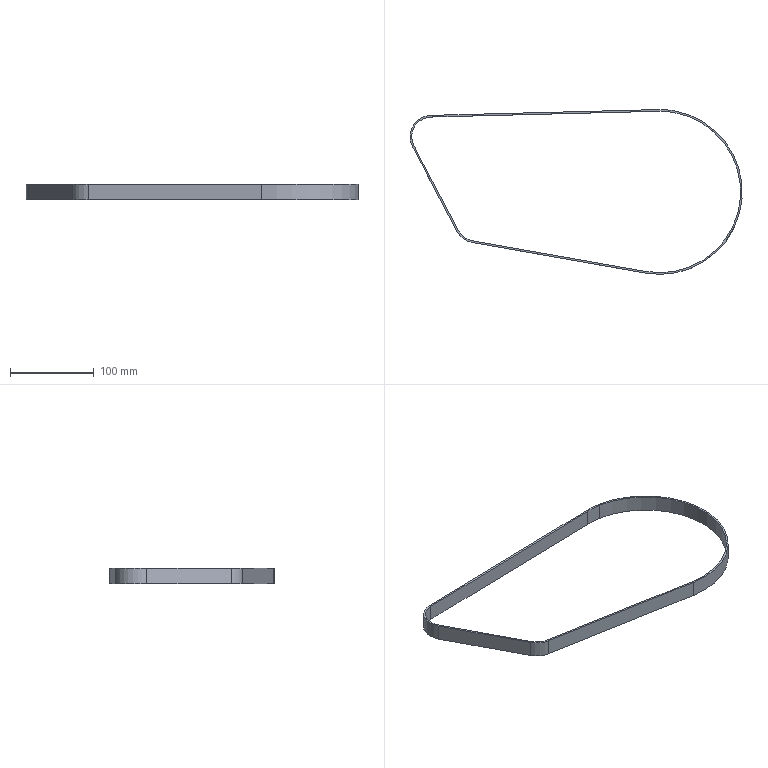Part | SolidWorks | features BaseBody 1 | 1 solid | 16 faces | box 396.622 x 196.734 x 19.05 mm | volume 38426 mm3 | cylinder 8 | plane 8 | commonest cylinder face diameters 47.139 x2 51.203 x2 192.67 x2 196.734 x2
STEP:
#1=CARTESIAN_POINT('',(270.213,30.425,-9.525));
#2=VERTEX_POINT('',#1);
#3=CARTESIAN_POINT('',(289.434,28.983,-9.525));
#4=VERTEX_POINT('',#3);
#5=CARTESIAN_POINT('',(272.654,-65.879,-9.525));
#6=DIRECTION('',(0.,0.,-1.));
#7=DIRECTION('',(0.1742,0.9847,0.));
#8=AXIS2_PLACEMENT_3D('',#5,#6,#7);
#9=CIRCLE('',#8,96.335);
#10=EDGE_CURVE('',#2,#4,#9,.T.);
#11=ORIENTED_EDGE('',*,*,#10,.T.);
#12=CARTESIAN_POINT('',(289.434,28.983,9.525));
#13=VERTEX_POINT('',#12);
#14=CARTESIAN_POINT('',(289.434,28.983,0.));
#15=DIRECTION('',(0.,0.,1.));
#16=VECTOR('',#15,1000.);
#17=LINE('',#14,#16);
#18=EDGE_CURVE('',#4,#13,#17,.T.);
#19=ORIENTED_EDGE('',*,*,#18,.T.);
#20=CARTESIAN_POINT('',(270.213,30.425,9.525));
#21=VERTEX_POINT('',#20);
#22=CARTESIAN_POINT('',(272.654,-65.879,9.525));
#23=DIRECTION('',(0.,0.,-1.));
#24=DIRECTION('',(0.1742,0.9847,0.));
#25=AXIS2_PLACEMENT_3D('',#22,#23,#24);
#26=CIRCLE('',#25,96.335);
#27=EDGE_CURVE('',#21,#13,#26,.T.);
#28=ORIENTED_EDGE('',*,*,#27,.F.);
#29=CARTESIAN_POINT('',(270.213,30.425,9.525));
#30=DIRECTION('',(0.,0.,1.));
#31=VECTOR('',#30,1000.);
#32=LINE('',#29,#31);
#33=EDGE_CURVE('',#2,#21,#32,.T.);
#34=ORIENTED_EDGE('',*,*,#33,.F.);
#35=EDGE_LOOP('',(#11,#19,#28,#34));
#36=FACE_OUTER_BOUND('',#35,.T.);
#37=CARTESIAN_POINT('',(272.654,-65.879,0.));
#38=DIRECTION('',(0.,0.,1.));
#39=DIRECTION('',(0.1742,0.9847,0.));
#40=AXIS2_PLACEMENT_3D('',#37,#38,#39);
#41=CYLINDRICAL_SURFACE('',#40,96.335);
#42=ADVANCED_FACE('',(#36),#41,.F.);
#43=CARTESIAN_POINT('',(289.788,30.984,-9.525));
#44=VERTEX_POINT('',#43);
#45=CARTESIAN_POINT('',(255.52,-162.742,-9.525));
#46=VERTEX_POINT('',#45);
#47=CARTESIAN_POINT('',(272.654,-65.879,-9.525));
#48=DIRECTION('',(0.,0.,-1.));
#49=DIRECTION('',(0.1742,0.9847,0.));
#50=AXIS2_PLACEMENT_3D('',#47,#48,#49);
#51=CIRCLE('',#50,98.367);
#52=EDGE_CURVE('',#44,#46,#51,.T.);
#53=ORIENTED_EDGE('',*,*,#52,.F.);
#54=CARTESIAN_POINT('',(289.788,30.984,9.525));
#55=VERTEX_POINT('',#54);
#56=CARTESIAN_POINT('',(289.788,30.984,0.));
#57=DIRECTION('',(0.,0.,1.));
#58=VECTOR('',#57,1000.);
#59=LINE('',#56,#58);
#60=EDGE_CURVE('',#44,#55,#59,.T.);
#61=ORIENTED_EDGE('',*,*,#60,.T.);
#62=CARTESIAN_POINT('',(255.52,-162.742,9.525));
#63=VERTEX_POINT('',#62);
#64=CARTESIAN_POINT('',(272.654,-65.879,9.525));
#65=DIRECTION('',(0.,0.,-1.));
#66=DIRECTION('',(0.1742,0.9847,0.));
#67=AXIS2_PLACEMENT_3D('',#64,#65,#66);
#68=CIRCLE('',#67,98.367);
#69=EDGE_CURVE('',#55,#63,#68,.T.);
#70=ORIENTED_EDGE('',*,*,#69,.T.);
#71=CARTESIAN_POINT('',(255.52,-162.742,-9.525));
#72=DIRECTION('',(0.,0.,1.));
#73=VECTOR('',#72,1000.);
#74=LINE('',#71,#73);
#75=EDGE_CURVE('',#46,#63,#74,.T.);
#76=ORIENTED_EDGE('',*,*,#75,.F.);
#77=EDGE_LOOP('',(#53,#61,#70,#76));
#78=FACE_OUTER_BOUND('',#77,.T.);
#79=CARTESIAN_POINT('',(272.654,-65.879,0.));
#80=DIRECTION('',(0.,0.,1.));
#81=DIRECTION('',(0.1742,0.9847,0.));
#82=AXIS2_PLACEMENT_3D('',#79,#80,#81);
#83=CYLINDRICAL_SURFACE('',#82,98.367);
#84=ADVANCED_FACE('',(#78),#83,.T.);
#85=ORIENTED_EDGE('',*,*,#33,.T.);
#86=CARTESIAN_POINT('',(-0.5971,23.562,9.525));
#87=VERTEX_POINT('',#86);
#88=CARTESIAN_POINT('',(-0.5971,23.562,9.525));
#89=DIRECTION('',(0.9997,0.02534,0.));
#90=VECTOR('',#89,1000.);
#91=LINE('',#88,#90);
#92=EDGE_CURVE('',#87,#21,#91,.T.);
#93=ORIENTED_EDGE('',*,*,#92,.F.);
#94=CARTESIAN_POINT('',(-0.5971,23.562,-9.525));
#95=VERTEX_POINT('',#94);
#96=CARTESIAN_POINT('',(-0.5971,23.562,9.525));
#97=DIRECTION('',(0.,0.,1.));
#98=VECTOR('',#97,1000.);
#99=LINE('',#96,#98);
#100=EDGE_CURVE('',#95,#87,#99,.T.);
#101=ORIENTED_EDGE('',*,*,#100,.F.);
#102=CARTESIAN_POINT('',(-0.5971,23.562,-9.525));
#103=DIRECTION('',(0.9997,0.02534,0.));
#104=VECTOR('',#103,1000.);
#105=LINE('',#102,#104);
#106=EDGE_CURVE('',#95,#2,#105,.T.);
#107=ORIENTED_EDGE('',*,*,#106,.T.);
#108=EDGE_LOOP('',(#85,#93,#101,#107));
#109=FACE_OUTER_BOUND('',#108,.T.);
#110=CARTESIAN_POINT('',(-0.5971,23.562,-9.525));
#111=DIRECTION('',(0.02534,-0.9997,0.));
#112=DIRECTION('',(0.,0.,-1.));
#113=AXIS2_PLACEMENT_3D('',#110,#111,#112);
#114=PLANE('',#113);
#115=ADVANCED_FACE('',(#109),#114,.T.);
#116=CARTESIAN_POINT('',(270.162,32.456,9.525));
#117=VERTEX_POINT('',#116);
#118=CARTESIAN_POINT('',(270.162,32.456,-9.525));
#119=VERTEX_POINT('',#118);
#120=CARTESIAN_POINT('',(270.162,32.456,-9.525));
#121=DIRECTION('',(0.,0.,-1.));
#122=VECTOR('',#121,1000.);
#123=LINE('',#120,#122);
#124=EDGE_CURVE('',#117,#119,#123,.T.);
#125=ORIENTED_EDGE('',*,*,#124,.T.);
#126=CARTESIAN_POINT('',(-0.6486,25.593,-9.525));
#127=VERTEX_POINT('',#126);
#128=CARTESIAN_POINT('',(-0.6486,25.593,-9.525));
#129=DIRECTION('',(0.9997,0.02534,0.));
#130=VECTOR('',#129,1000.);
#131=LINE('',#128,#130);
#132=EDGE_CURVE('',#127,#119,#131,.T.);
#133=ORIENTED_EDGE('',*,*,#132,.F.);
#134=CARTESIAN_POINT('',(-0.6486,25.593,9.525));
#135=VERTEX_POINT('',#134);
#136=CARTESIAN_POINT('',(-0.6486,25.593,-9.525));
#137=DIRECTION('',(0.,0.,-1.));
#138=VECTOR('',#137,1000.);
#139=LINE('',#136,#138);
#140=EDGE_CURVE('',#135,#127,#139,.T.);
#141=ORIENTED_EDGE('',*,*,#140,.F.);
#142=CARTESIAN_POINT('',(-0.6486,25.593,9.525));
#143=DIRECTION('',(0.9997,0.02534,0.));
#144=VECTOR('',#143,1000.);
#145=LINE('',#142,#144);
#146=EDGE_CURVE('',#135,#117,#145,.T.);
#147=ORIENTED_EDGE('',*,*,#146,.T.);
#148=EDGE_LOOP('',(#125,#133,#141,#147));
#149=FACE_OUTER_BOUND('',#148,.T.);
#150=CARTESIAN_POINT('',(-0.6486,25.593,9.525));
#151=DIRECTION('',(-0.02534,0.9997,0.));
#152=DIRECTION('',(0.,0.,1.));
#153=AXIS2_PLACEMENT_3D('',#150,#151,#152);
#154=PLANE('',#153);
#155=ADVANCED_FACE('',(#149),#154,.T.);
#156=ORIENTED_EDGE('',*,*,#100,.T.);
#157=CARTESIAN_POINT('',(-20.854,-10.982,9.525));
#158=VERTEX_POINT('',#157);
#159=CARTESIAN_POINT('',(0.,0.,9.525));
#160=DIRECTION('',(0.,0.,-1.));
#161=DIRECTION('',(0.02534,-0.9997,0.));
#162=AXIS2_PLACEMENT_3D('',#159,#160,#161);
#163=CIRCLE('',#162,23.569);
#164=EDGE_CURVE('',#158,#87,#163,.T.);
#165=ORIENTED_EDGE('',*,*,#164,.F.);
#166=CARTESIAN_POINT('',(-20.854,-10.982,-9.525));
#167=VERTEX_POINT('',#166);
#168=CARTESIAN_POINT('',(-20.854,-10.982,9.525));
#169=DIRECTION('',(0.,0.,1.));
#170=VECTOR('',#169,1000.);
#171=LINE('',#168,#170);
#172=EDGE_CURVE('',#167,#158,#171,.T.);
#173=ORIENTED_EDGE('',*,*,#172,.F.);
#174=CARTESIAN_POINT('',(0.,0.,-9.525));
#175=DIRECTION('',(0.,0.,-1.));
#176=DIRECTION('',(0.02534,-0.9997,0.));
#177=AXIS2_PLACEMENT_3D('',#174,#175,#176);
#178=CIRCLE('',#177,23.569);
#179=EDGE_CURVE('',#167,#95,#178,.T.);
#180=ORIENTED_EDGE('',*,*,#179,.T.);
#181=EDGE_LOOP('',(#156,#165,#173,#180));
#182=FACE_OUTER_BOUND('',#181,.T.);
#183=CARTESIAN_POINT('',(0.,0.,0.));
#184=DIRECTION('',(0.,0.,1.));
#185=DIRECTION('',(0.02534,-0.9997,0.));
#186=AXIS2_PLACEMENT_3D('',#183,#184,#185);
#187=CYLINDRICAL_SURFACE('',#186,23.569);
#188=ADVANCED_FACE('',(#182),#187,.F.);
#189=ORIENTED_EDGE('',*,*,#140,.T.);
#190=CARTESIAN_POINT('',(-22.652,-11.929,-9.525));
#191=VERTEX_POINT('',#190);
#192=CARTESIAN_POINT('',(0.,0.,-9.525));
#193=DIRECTION('',(0.,0.,-1.));
#194=DIRECTION('',(0.02534,-0.9997,0.));
#195=AXIS2_PLACEMENT_3D('',#192,#193,#194);
#196=CIRCLE('',#195,25.601);
#197=EDGE_CURVE('',#191,#127,#196,.T.);
#198=ORIENTED_EDGE('',*,*,#197,.F.);
#199=CARTESIAN_POINT('',(-22.652,-11.929,9.525));
#200=VERTEX_POINT('',#199);
#201=CARTESIAN_POINT('',(-22.652,-11.929,-9.525));
#202=DIRECTION('',(0.,0.,-1.));
#203=VECTOR('',#202,1000.);
#204=LINE('',#201,#203);
#205=EDGE_CURVE('',#200,#191,#204,.T.);
#206=ORIENTED_EDGE('',*,*,#205,.F.);
#207=CARTESIAN_POINT('',(0.,0.,9.525));
#208=DIRECTION('',(0.,0.,-1.));
#209=DIRECTION('',(0.02534,-0.9997,0.));
#210=AXIS2_PLACEMENT_3D('',#207,#208,#209);
#211=CIRCLE('',#210,25.601);
#212=EDGE_CURVE('',#200,#135,#211,.T.);
#213=ORIENTED_EDGE('',*,*,#212,.T.);
#214=EDGE_LOOP('',(#189,#198,#206,#213));
#215=FACE_OUTER_BOUND('',#214,.T.);
#216=CARTESIAN_POINT('',(0.,0.,0.));
#217=DIRECTION('',(0.,0.,1.));
#218=DIRECTION('',(0.02534,-0.9997,0.));
#219=AXIS2_PLACEMENT_3D('',#216,#217,#218);
#220=CYLINDRICAL_SURFACE('',#219,25.601);
#221=ADVANCED_FACE('',(#215),#220,.T.);
#222=ORIENTED_EDGE('',*,*,#172,.T.);
#223=CARTESIAN_POINT('',(32.307,-111.93,9.525));
#224=VERTEX_POINT('',#223);
#225=CARTESIAN_POINT('',(32.307,-111.93,9.525));
#226=DIRECTION('',(-0.466,0.8848,0.));
#227=VECTOR('',#226,1000.);
#228=LINE('',#225,#227);
#229=EDGE_CURVE('',#224,#158,#228,.T.);
#230=ORIENTED_EDGE('',*,*,#229,.F.);
#231=CARTESIAN_POINT('',(32.307,-111.93,-9.525));
#232=VERTEX_POINT('',#231);
#233=CARTESIAN_POINT('',(32.307,-111.93,9.525));
#234=DIRECTION('',(0.,0.,1.));
#235=VECTOR('',#234,1000.);
#236=LINE('',#233,#235);
#237=EDGE_CURVE('',#232,#224,#236,.T.);
#238=ORIENTED_EDGE('',*,*,#237,.F.);
#239=CARTESIAN_POINT('',(32.307,-111.93,-9.525));
#240=DIRECTION('',(-0.466,0.8848,0.));
#241=VECTOR('',#240,1000.);
#242=LINE('',#239,#241);
#243=EDGE_CURVE('',#232,#167,#242,.T.);
#244=ORIENTED_EDGE('',*,*,#243,.T.);
#245=EDGE_LOOP('',(#222,#230,#238,#244));
#246=FACE_OUTER_BOUND('',#245,.T.);
#247=CARTESIAN_POINT('',(32.307,-111.93,-9.525));
#248=DIRECTION('',(0.8848,0.466,0.));
#249=DIRECTION('',(0.,0.,-1.));
#250=AXIS2_PLACEMENT_3D('',#247,#248,#249);
#251=PLANE('',#250);
#252=ADVANCED_FACE('',(#246),#251,.T.);
#253=ORIENTED_EDGE('',*,*,#205,.T.);
#254=CARTESIAN_POINT('',(30.509,-112.877,-9.525));
#255=VERTEX_POINT('',#254);
#256=CARTESIAN_POINT('',(30.509,-112.877,-9.525));
#257=DIRECTION('',(-0.466,0.8848,0.));
#258=VECTOR('',#257,1000.);
#259=LINE('',#256,#258);
#260=EDGE_CURVE('',#255,#191,#259,.T.);
#261=ORIENTED_EDGE('',*,*,#260,.F.);
#262=CARTESIAN_POINT('',(30.509,-112.877,9.525));
#263=VERTEX_POINT('',#262);
#264=CARTESIAN_POINT('',(30.509,-112.877,-9.525));
#265=DIRECTION('',(0.,0.,-1.));
#266=VECTOR('',#265,1000.);
#267=LINE('',#264,#266);
#268=EDGE_CURVE('',#263,#255,#267,.T.);
#269=ORIENTED_EDGE('',*,*,#268,.F.);
#270=CARTESIAN_POINT('',(30.509,-112.877,9.525));
#271=DIRECTION('',(-0.466,0.8848,0.));
#272=VECTOR('',#271,1000.);
#273=LINE('',#270,#272);
#274=EDGE_CURVE('',#263,#200,#273,.T.);
#275=ORIENTED_EDGE('',*,*,#274,.T.);
#276=EDGE_LOOP('',(#253,#261,#269,#275));
#277=FACE_OUTER_BOUND('',#276,.T.);
#278=CARTESIAN_POINT('',(30.509,-112.877,9.525));
#279=DIRECTION('',(-0.8848,-0.466,0.));
#280=DIRECTION('',(-0.466,0.8848,0.));
#281=AXIS2_PLACEMENT_3D('',#278,#279,#280);
#282=PLANE('',#281);
#283=ADVANCED_FACE('',(#277),#282,.T.);
#284=CARTESIAN_POINT('',(255.874,-160.741,-9.525));
#285=VERTEX_POINT('',#284);
#286=CARTESIAN_POINT('',(49.056,-124.157,-9.525));
#287=VERTEX_POINT('',#286);
#288=CARTESIAN_POINT('',(255.874,-160.741,-9.525));
#289=DIRECTION('',(-0.9847,0.1742,0.));
#290=VECTOR('',#289,1000.);
#291=LINE('',#288,#290);
#292=EDGE_CURVE('',#285,#287,#291,.T.);
#293=ORIENTED_EDGE('',*,*,#292,.F.);
#294=CARTESIAN_POINT('',(272.654,-65.879,-9.525));
#295=DIRECTION('',(0.,0.,-1.));
#296=DIRECTION('',(0.1742,0.9847,0.));
#297=AXIS2_PLACEMENT_3D('',#294,#295,#296);
#298=CIRCLE('',#297,96.335);
#299=EDGE_CURVE('',#4,#285,#298,.T.);
#300=ORIENTED_EDGE('',*,*,#299,.F.);
#301=ORIENTED_EDGE('',*,*,#10,.F.);
#302=ORIENTED_EDGE('',*,*,#106,.F.);
#303=ORIENTED_EDGE('',*,*,#179,.F.);
#304=ORIENTED_EDGE('',*,*,#243,.F.);
#305=CARTESIAN_POINT('',(53.161,-100.948,-9.525));
#306=DIRECTION('',(0.,0.,-1.));
#307=DIRECTION('',(0.8848,0.466,0.));
#308=AXIS2_PLACEMENT_3D('',#305,#306,#307);
#309=CIRCLE('',#308,23.569);
#310=EDGE_CURVE('',#287,#232,#309,.T.);
#311=ORIENTED_EDGE('',*,*,#310,.F.);
#312=EDGE_LOOP('',(#293,#300,#301,#302,#303,#304,#311));
#313=FACE_BOUND('',#312,.T.);
#314=CARTESIAN_POINT('',(48.702,-126.158,-9.525));
#315=VERTEX_POINT('',#314);
#316=CARTESIAN_POINT('',(53.161,-100.948,-9.525));
#317=DIRECTION('',(0.,0.,-1.));
#318=DIRECTION('',(0.8848,0.466,0.));
#319=AXIS2_PLACEMENT_3D('',#316,#317,#318);
#320=CIRCLE('',#319,25.601);
#321=EDGE_CURVE('',#315,#255,#320,.T.);
#322=ORIENTED_EDGE('',*,*,#321,.T.);
#323=ORIENTED_EDGE('',*,*,#260,.T.);
#324=ORIENTED_EDGE('',*,*,#197,.T.);
#325=ORIENTED_EDGE('',*,*,#132,.T.);
#326=CARTESIAN_POINT('',(272.654,-65.879,-9.525));
#327=DIRECTION('',(0.,0.,-1.));
#328=DIRECTION('',(0.1742,0.9847,0.));
#329=AXIS2_PLACEMENT_3D('',#326,#327,#328);
#330=CIRCLE('',#329,98.367);
#331=EDGE_CURVE('',#119,#44,#330,.T.);
#332=ORIENTED_EDGE('',*,*,#331,.T.);
#333=ORIENTED_EDGE('',*,*,#52,.T.);
#334=CARTESIAN_POINT('',(255.52,-162.742,-9.525));
#335=DIRECTION('',(-0.9847,0.1742,0.));
#336=VECTOR('',#335,1000.);
#337=LINE('',#334,#336);
#338=EDGE_CURVE('',#46,#315,#337,.T.);
#339=ORIENTED_EDGE('',*,*,#338,.T.);
#340=EDGE_LOOP('',(#322,#323,#324,#325,#332,#333,#339));
#341=FACE_OUTER_BOUND('',#340,.T.);
#342=CARTESIAN_POINT('',(48.879,-125.157,-9.525));
#343=DIRECTION('',(0.,0.,-1.));
#344=DIRECTION('',(0.,-1.,0.));
#345=AXIS2_PLACEMENT_3D('',#342,#343,#344);
#346=PLANE('',#345);
#347=ADVANCED_FACE('',(#313,#341),#346,.T.);
#348=ORIENTED_EDGE('',*,*,#237,.T.);
#349=CARTESIAN_POINT('',(49.056,-124.157,9.525));
#350=VERTEX_POINT('',#349);
#351=CARTESIAN_POINT('',(53.161,-100.948,9.525));
#352=DIRECTION('',(0.,0.,-1.));
#353=DIRECTION('',(0.8848,0.466,0.));
#354=AXIS2_PLACEMENT_3D('',#351,#352,#353);
#355=CIRCLE('',#354,23.569);
#356=EDGE_CURVE('',#350,#224,#355,.T.);
#357=ORIENTED_EDGE('',*,*,#356,.F.);
#358=CARTESIAN_POINT('',(49.056,-124.157,9.525));
#359=DIRECTION('',(0.,0.,1.));
#360=VECTOR('',#359,1000.);
#361=LINE('',#358,#360);
#362=EDGE_CURVE('',#287,#350,#361,.T.);
#363=ORIENTED_EDGE('',*,*,#362,.F.);
#364=ORIENTED_EDGE('',*,*,#310,.T.);
#365=EDGE_LOOP('',(#348,#357,#363,#364));
#366=FACE_OUTER_BOUND('',#365,.T.);
#367=CARTESIAN_POINT('',(53.161,-100.948,0.));
#368=DIRECTION('',(0.,0.,1.));
#369=DIRECTION('',(0.8848,0.466,0.));
#370=AXIS2_PLACEMENT_3D('',#367,#368,#369);
#371=CYLINDRICAL_SURFACE('',#370,23.569);
#372=ADVANCED_FACE('',(#366),#371,.F.);
#373=ORIENTED_EDGE('',*,*,#356,.T.);
#374=ORIENTED_EDGE('',*,*,#229,.T.);
#375=ORIENTED_EDGE('',*,*,#164,.T.);
#376=ORIENTED_EDGE('',*,*,#92,.T.);
#377=ORIENTED_EDGE('',*,*,#27,.T.);
#378=CARTESIAN_POINT('',(255.874,-160.741,9.525));
#379=VERTEX_POINT('',#378);
#380=CARTESIAN_POINT('',(272.654,-65.879,9.525));
#381=DIRECTION('',(0.,0.,-1.));
#382=DIRECTION('',(0.1742,0.9847,0.));
#383=AXIS2_PLACEMENT_3D('',#380,#381,#382);
#384=CIRCLE('',#383,96.335);
#385=EDGE_CURVE('',#13,#379,#384,.T.);
#386=ORIENTED_EDGE('',*,*,#385,.T.);
#387=CARTESIAN_POINT('',(255.874,-160.741,9.525));
#388=DIRECTION('',(-0.9847,0.1742,0.));
#389=VECTOR('',#388,1000.);
#390=LINE('',#387,#389);
#391=EDGE_CURVE('',#379,#350,#390,.T.);
#392=ORIENTED_EDGE('',*,*,#391,.T.);
#393=EDGE_LOOP('',(#373,#374,#375,#376,#377,#386,#392));
#394=FACE_BOUND('',#393,.T.);
#395=CARTESIAN_POINT('',(48.702,-126.158,9.525));
#396=VERTEX_POINT('',#395);
#397=CARTESIAN_POINT('',(255.52,-162.742,9.525));
#398=DIRECTION('',(-0.9847,0.1742,0.));
#399=VECTOR('',#398,1000.);
#400=LINE('',#397,#399);
#401=EDGE_CURVE('',#63,#396,#400,.T.);
#402=ORIENTED_EDGE('',*,*,#401,.F.);
#403=ORIENTED_EDGE('',*,*,#69,.F.);
#404=CARTESIAN_POINT('',(272.654,-65.879,9.525));
#405=DIRECTION('',(0.,0.,-1.));
#406=DIRECTION('',(0.1742,0.9847,0.));
#407=AXIS2_PLACEMENT_3D('',#404,#405,#406);
#408=CIRCLE('',#407,98.367);
#409=EDGE_CURVE('',#117,#55,#408,.T.);
#410=ORIENTED_EDGE('',*,*,#409,.F.);
#411=ORIENTED_EDGE('',*,*,#146,.F.);
#412=ORIENTED_EDGE('',*,*,#212,.F.);
#413=ORIENTED_EDGE('',*,*,#274,.F.);
#414=CARTESIAN_POINT('',(53.161,-100.948,9.525));
#415=DIRECTION('',(0.,0.,-1.));
#416=DIRECTION('',(0.8848,0.466,0.));
#417=AXIS2_PLACEMENT_3D('',#414,#415,#416);
#418=CIRCLE('',#417,25.601);
#419=EDGE_CURVE('',#396,#263,#418,.T.);
#420=ORIENTED_EDGE('',*,*,#419,.F.);
#421=EDGE_LOOP('',(#402,#403,#410,#411,#412,#413,#420));
#422=FACE_OUTER_BOUND('',#421,.T.);
#423=CARTESIAN_POINT('',(48.879,-125.157,9.525));
#424=DIRECTION('',(0.,0.,1.));
#425=DIRECTION('',(1.,0.,0.));
#426=AXIS2_PLACEMENT_3D('',#423,#424,#425);
#427=PLANE('',#426);
#428=ADVANCED_FACE('',(#394,#422),#427,.T.);
#429=ORIENTED_EDGE('',*,*,#268,.T.);
#430=ORIENTED_EDGE('',*,*,#321,.F.);
#431=CARTESIAN_POINT('',(48.702,-126.158,-9.525));
#432=DIRECTION('',(0.,0.,-1.));
#433=VECTOR('',#432,1000.);
#434=LINE('',#431,#433);
#435=EDGE_CURVE('',#396,#315,#434,.T.);
#436=ORIENTED_EDGE('',*,*,#435,.F.);
#437=ORIENTED_EDGE('',*,*,#419,.T.);
#438=EDGE_LOOP('',(#429,#430,#436,#437));
#439=FACE_OUTER_BOUND('',#438,.T.);
#440=CARTESIAN_POINT('',(53.161,-100.948,0.));
#441=DIRECTION('',(0.,0.,1.));
#442=DIRECTION('',(0.8848,0.466,0.));
#443=AXIS2_PLACEMENT_3D('',#440,#441,#442);
#444=CYLINDRICAL_SURFACE('',#443,25.601);
#445=ADVANCED_FACE('',(#439),#444,.T.);
#446=ORIENTED_EDGE('',*,*,#362,.T.);
#447=ORIENTED_EDGE('',*,*,#391,.F.);
#448=CARTESIAN_POINT('',(255.874,-160.741,9.525));
#449=DIRECTION('',(0.,0.,-1.));
#450=VECTOR('',#449,1000.);
#451=LINE('',#448,#450);
#452=EDGE_CURVE('',#379,#285,#451,.T.);
#453=ORIENTED_EDGE('',*,*,#452,.T.);
#454=ORIENTED_EDGE('',*,*,#292,.T.);
#455=EDGE_LOOP('',(#446,#447,#453,#454));
#456=FACE_OUTER_BOUND('',#455,.T.);
#457=CARTESIAN_POINT('',(255.874,-160.741,-9.525));
#458=DIRECTION('',(0.1742,0.9847,0.));
#459=DIRECTION('',(0.,0.,-1.));
#460=AXIS2_PLACEMENT_3D('',#457,#458,#459);
#461=PLANE('',#460);
#462=ADVANCED_FACE('',(#456),#461,.T.);
#463=ORIENTED_EDGE('',*,*,#435,.T.);
#464=ORIENTED_EDGE('',*,*,#338,.F.);
#465=ORIENTED_EDGE('',*,*,#75,.T.);
#466=ORIENTED_EDGE('',*,*,#401,.T.);
#467=EDGE_LOOP('',(#463,#464,#465,#466));
#468=FACE_OUTER_BOUND('',#467,.T.);
#469=CARTESIAN_POINT('',(255.52,-162.742,9.525));
#470=DIRECTION('',(-0.1742,-0.9847,0.));
#471=DIRECTION('',(-0.9847,0.1742,0.));
#472=AXIS2_PLACEMENT_3D('',#469,#470,#471);
#473=PLANE('',#472);
#474=ADVANCED_FACE('',(#468),#473,.T.);
#475=ORIENTED_EDGE('',*,*,#60,.F.);
#476=ORIENTED_EDGE('',*,*,#331,.F.);
#477=ORIENTED_EDGE('',*,*,#124,.F.);
#478=ORIENTED_EDGE('',*,*,#409,.T.);
#479=EDGE_LOOP('',(#475,#476,#477,#478));
#480=FACE_OUTER_BOUND('',#479,.T.);
#481=CARTESIAN_POINT('',(272.654,-65.879,0.));
#482=DIRECTION('',(0.,0.,1.));
#483=DIRECTION('',(0.1742,0.9847,0.));
#484=AXIS2_PLACEMENT_3D('',#481,#482,#483);
#485=CYLINDRICAL_SURFACE('',#484,98.367);
#486=ADVANCED_FACE('',(#480),#485,.T.);
#487=ORIENTED_EDGE('',*,*,#18,.F.);
#488=ORIENTED_EDGE('',*,*,#299,.T.);
#489=ORIENTED_EDGE('',*,*,#452,.F.);
#490=ORIENTED_EDGE('',*,*,#385,.F.);
#491=EDGE_LOOP('',(#487,#488,#489,#490));
#492=FACE_OUTER_BOUND('',#491,.T.);
#493=CARTESIAN_POINT('',(272.654,-65.879,0.));
#494=DIRECTION('',(0.,0.,1.));
#495=DIRECTION('',(0.1742,0.9847,0.));
#496=AXIS2_PLACEMENT_3D('',#493,#494,#495);
#497=CYLINDRICAL_SURFACE('',#496,96.335);
#498=ADVANCED_FACE('',(#492),#497,.F.);
#499=CLOSED_SHELL('',(#42,#84,#115,#155,#188,#221,#252,#283,#347,#372,#428,#445,#462,#474,#486,#498));
#500=MANIFOLD_SOLID_BREP('',#499);
#501=CARTESIAN_POINT('',(0.,0.,0.));
#502=DIRECTION('',(0.,0.,1.));
#503=DIRECTION('',(1.,0.,0.));
#504=AXIS2_PLACEMENT_3D('',#501,#502,#503);
#505=(LENGTH_UNIT()NAMED_UNIT(*)SI_UNIT(.MILLI.,.METRE.));
#506=UNCERTAINTY_MEASURE_WITH_UNIT(LENGTH_MEASURE(0.00001),#505,'','');
#507=(NAMED_UNIT(*)PLANE_ANGLE_UNIT()SI_UNIT($,.RADIAN.));
#508=(NAMED_UNIT(*)SI_UNIT($,.STERADIAN.)SOLID_ANGLE_UNIT());
#509=(GEOMETRIC_REPRESENTATION_CONTEXT(3)GLOBAL_UNCERTAINTY_ASSIGNED_CONTEXT((#506))GLOBAL_UNIT_ASSIGNED_CONTEXT((#505,#507,#508))REPRESENTATION_CONTEXT('',''));
#510=ADVANCED_BREP_SHAPE_REPRESENTATION('',(#500,#504),#509);